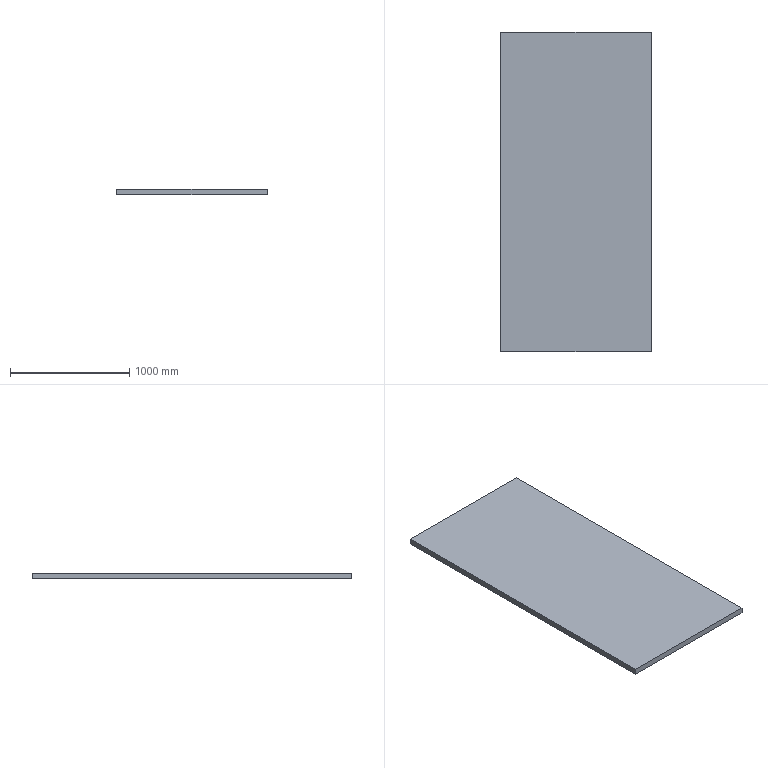Part | STEP file | 1 solid | 6 faces | box 1260 x 2677 x 50 mm | volume 168683678 mm3 | plane 6
STEP:
#1=CARTESIAN_POINT('',(0.,0.,0.));
#2=DIRECTION('',(0.,0.,1.));
#3=DIRECTION('',(1.,0.,0.));
#4=AXIS2_PLACEMENT_3D('',#1,#2,#3);
#5=CARTESIAN_POINT('',(6051.871,-1690.161,-25.));
#6=VERTEX_POINT('',#5);
#7=CARTESIAN_POINT('',(6051.871,986.805,-25.));
#8=VERTEX_POINT('',#7);
#9=CARTESIAN_POINT('',(6051.871,986.805,-25.));
#10=DIRECTION('',(0.,1.,0.));
#11=VECTOR('',#10,1.);
#12=LINE('',#9,#11);
#13=CARTESIAN_POINT('',(6051.871,986.805,25.));
#14=DIRECTION('',(-1.,0.,0.));
#15=DIRECTION('',(0.,0.,1.));
#16=AXIS2_PLACEMENT_3D('',#13,#14,#15);
#17=PLANE('',#16);
#18=CARTESIAN_POINT('',(-50.,0.));
#19=DIRECTION('',(0.,1.));
#20=VECTOR('',#19,1.);
#21=LINE('',#18,#20);
#22=(GEOMETRIC_REPRESENTATION_CONTEXT(2)PARAMETRIC_REPRESENTATION_CONTEXT()REPRESENTATION_CONTEXT('',''));
#23=DEFINITIONAL_REPRESENTATION('',(#21),#22);
#24=PCURVE('',#17,#23);
#25=CARTESIAN_POINT('',(0.,0.,-25.));
#26=DIRECTION('',(0.,0.,-1.));
#27=DIRECTION('',(-1.,0.,0.));
#28=AXIS2_PLACEMENT_3D('',#25,#26,#27);
#29=PLANE('',#28);
#30=CARTESIAN_POINT('',(-6051.871,986.805));
#31=DIRECTION('',(0.,1.));
#32=VECTOR('',#31,1.);
#33=LINE('',#30,#32);
#34=(GEOMETRIC_REPRESENTATION_CONTEXT(2)PARAMETRIC_REPRESENTATION_CONTEXT()REPRESENTATION_CONTEXT('',''));
#35=DEFINITIONAL_REPRESENTATION('',(#33),#34);
#36=PCURVE('',#29,#35);
#37=SURFACE_CURVE('',#12,(#24,#36),.PCURVE_S1.);
#38=EDGE_CURVE('',#6,#8,#37,.T.);
#39=ORIENTED_EDGE('',*,*,#38,.T.);
#40=CARTESIAN_POINT('',(6051.871,986.805,25.));
#41=VERTEX_POINT('',#40);
#42=CARTESIAN_POINT('',(6051.871,986.805,25.));
#43=DIRECTION('',(0.,0.,-1.));
#44=VECTOR('',#43,1.);
#45=LINE('',#42,#44);
#46=CARTESIAN_POINT('',(0.,0.));
#47=DIRECTION('',(-1.,0.));
#48=VECTOR('',#47,1.);
#49=LINE('',#46,#48);
#50=(GEOMETRIC_REPRESENTATION_CONTEXT(2)PARAMETRIC_REPRESENTATION_CONTEXT()REPRESENTATION_CONTEXT('',''));
#51=DEFINITIONAL_REPRESENTATION('',(#49),#50);
#52=PCURVE('',#17,#51);
#53=CARTESIAN_POINT('',(6051.871,986.805,25.));
#54=DIRECTION('',(0.,-1.,0.));
#55=DIRECTION('',(0.,0.,-1.));
#56=AXIS2_PLACEMENT_3D('',#53,#54,#55);
#57=PLANE('',#56);
#58=CARTESIAN_POINT('',(0.,0.));
#59=DIRECTION('',(1.,0.));
#60=VECTOR('',#59,1.);
#61=LINE('',#58,#60);
#62=(GEOMETRIC_REPRESENTATION_CONTEXT(2)PARAMETRIC_REPRESENTATION_CONTEXT()REPRESENTATION_CONTEXT('',''));
#63=DEFINITIONAL_REPRESENTATION('',(#61),#62);
#64=PCURVE('',#57,#63);
#65=SURFACE_CURVE('',#45,(#52,#64),.PCURVE_S1.);
#66=EDGE_CURVE('',#41,#8,#65,.T.);
#67=ORIENTED_EDGE('',*,*,#66,.F.);
#68=CARTESIAN_POINT('',(6051.871,-1690.161,25.));
#69=VERTEX_POINT('',#68);
#70=CARTESIAN_POINT('',(6051.871,986.805,25.));
#71=DIRECTION('',(0.,1.,0.));
#72=VECTOR('',#71,1.);
#73=LINE('',#70,#72);
#74=CARTESIAN_POINT('',(0.,0.));
#75=DIRECTION('',(0.,1.));
#76=VECTOR('',#75,1.);
#77=LINE('',#74,#76);
#78=(GEOMETRIC_REPRESENTATION_CONTEXT(2)PARAMETRIC_REPRESENTATION_CONTEXT()REPRESENTATION_CONTEXT('',''));
#79=DEFINITIONAL_REPRESENTATION('',(#77),#78);
#80=PCURVE('',#17,#79);
#81=CARTESIAN_POINT('',(0.,0.,25.));
#82=DIRECTION('',(0.,0.,-1.));
#83=DIRECTION('',(-1.,0.,0.));
#84=AXIS2_PLACEMENT_3D('',#81,#82,#83);
#85=PLANE('',#84);
#86=CARTESIAN_POINT('',(-6051.871,986.805));
#87=DIRECTION('',(0.,1.));
#88=VECTOR('',#87,1.);
#89=LINE('',#86,#88);
#90=(GEOMETRIC_REPRESENTATION_CONTEXT(2)PARAMETRIC_REPRESENTATION_CONTEXT()REPRESENTATION_CONTEXT('',''));
#91=DEFINITIONAL_REPRESENTATION('',(#89),#90);
#92=PCURVE('',#85,#91);
#93=SURFACE_CURVE('',#73,(#80,#92),.PCURVE_S1.);
#94=EDGE_CURVE('',#69,#41,#93,.T.);
#95=ORIENTED_EDGE('',*,*,#94,.F.);
#96=CARTESIAN_POINT('',(6051.871,-1690.161,25.));
#97=DIRECTION('',(0.,0.,-1.));
#98=VECTOR('',#97,1.);
#99=LINE('',#96,#98);
#100=CARTESIAN_POINT('',(0.,-2676.966));
#101=DIRECTION('',(-1.,0.));
#102=VECTOR('',#101,1.);
#103=LINE('',#100,#102);
#104=(GEOMETRIC_REPRESENTATION_CONTEXT(2)PARAMETRIC_REPRESENTATION_CONTEXT()REPRESENTATION_CONTEXT('',''));
#105=DEFINITIONAL_REPRESENTATION('',(#103),#104);
#106=PCURVE('',#17,#105);
#107=CARTESIAN_POINT('',(6051.871,-1690.161,25.));
#108=DIRECTION('',(0.,1.,0.));
#109=DIRECTION('',(0.,0.,1.));
#110=AXIS2_PLACEMENT_3D('',#107,#108,#109);
#111=PLANE('',#110);
#112=CARTESIAN_POINT('',(0.,0.));
#113=DIRECTION('',(-1.,0.));
#114=VECTOR('',#113,1.);
#115=LINE('',#112,#114);
#116=(GEOMETRIC_REPRESENTATION_CONTEXT(2)PARAMETRIC_REPRESENTATION_CONTEXT()REPRESENTATION_CONTEXT('',''));
#117=DEFINITIONAL_REPRESENTATION('',(#115),#116);
#118=PCURVE('',#111,#117);
#119=SURFACE_CURVE('',#99,(#106,#118),.PCURVE_S1.);
#120=EDGE_CURVE('',#69,#6,#119,.T.);
#121=ORIENTED_EDGE('',*,*,#120,.T.);
#122=EDGE_LOOP('',(#39,#67,#95,#121));
#123=FACE_BOUND('',#122,.T.);
#124=ADVANCED_FACE('',(#123),#17,.F.);
#125=CARTESIAN_POINT('',(4791.611,986.805,-25.));
#126=VERTEX_POINT('',#125);
#127=CARTESIAN_POINT('',(6051.871,986.805,-25.));
#128=DIRECTION('',(-1.,0.,0.));
#129=VECTOR('',#128,1.);
#130=LINE('',#127,#129);
#131=CARTESIAN_POINT('',(50.,0.));
#132=DIRECTION('',(0.,-1.));
#133=VECTOR('',#132,1.);
#134=LINE('',#131,#133);
#135=(GEOMETRIC_REPRESENTATION_CONTEXT(2)PARAMETRIC_REPRESENTATION_CONTEXT()REPRESENTATION_CONTEXT('',''));
#136=DEFINITIONAL_REPRESENTATION('',(#134),#135);
#137=PCURVE('',#57,#136);
#138=CARTESIAN_POINT('',(-6051.871,986.805));
#139=DIRECTION('',(1.,0.));
#140=VECTOR('',#139,1.);
#141=LINE('',#138,#140);
#142=(GEOMETRIC_REPRESENTATION_CONTEXT(2)PARAMETRIC_REPRESENTATION_CONTEXT()REPRESENTATION_CONTEXT('',''));
#143=DEFINITIONAL_REPRESENTATION('',(#141),#142);
#144=PCURVE('',#29,#143);
#145=SURFACE_CURVE('',#130,(#137,#144),.PCURVE_S1.);
#146=EDGE_CURVE('',#8,#126,#145,.T.);
#147=ORIENTED_EDGE('',*,*,#146,.T.);
#148=CARTESIAN_POINT('',(4791.611,986.805,25.));
#149=VERTEX_POINT('',#148);
#150=CARTESIAN_POINT('',(4791.611,986.805,25.));
#151=DIRECTION('',(0.,0.,-1.));
#152=VECTOR('',#151,1.);
#153=LINE('',#150,#152);
#154=CARTESIAN_POINT('',(0.,-1260.26));
#155=DIRECTION('',(1.,0.));
#156=VECTOR('',#155,1.);
#157=LINE('',#154,#156);
#158=(GEOMETRIC_REPRESENTATION_CONTEXT(2)PARAMETRIC_REPRESENTATION_CONTEXT()REPRESENTATION_CONTEXT('',''));
#159=DEFINITIONAL_REPRESENTATION('',(#157),#158);
#160=PCURVE('',#57,#159);
#161=CARTESIAN_POINT('',(4791.611,986.805,25.));
#162=DIRECTION('',(1.,0.,0.));
#163=DIRECTION('',(0.,0.,-1.));
#164=AXIS2_PLACEMENT_3D('',#161,#162,#163);
#165=PLANE('',#164);
#166=CARTESIAN_POINT('',(0.,0.));
#167=DIRECTION('',(1.,0.));
#168=VECTOR('',#167,1.);
#169=LINE('',#166,#168);
#170=(GEOMETRIC_REPRESENTATION_CONTEXT(2)PARAMETRIC_REPRESENTATION_CONTEXT()REPRESENTATION_CONTEXT('',''));
#171=DEFINITIONAL_REPRESENTATION('',(#169),#170);
#172=PCURVE('',#165,#171);
#173=SURFACE_CURVE('',#153,(#160,#172),.PCURVE_S1.);
#174=EDGE_CURVE('',#149,#126,#173,.T.);
#175=ORIENTED_EDGE('',*,*,#174,.F.);
#176=CARTESIAN_POINT('',(6051.871,986.805,25.));
#177=DIRECTION('',(-1.,0.,0.));
#178=VECTOR('',#177,1.);
#179=LINE('',#176,#178);
#180=CARTESIAN_POINT('',(0.,0.));
#181=DIRECTION('',(0.,-1.));
#182=VECTOR('',#181,1.);
#183=LINE('',#180,#182);
#184=(GEOMETRIC_REPRESENTATION_CONTEXT(2)PARAMETRIC_REPRESENTATION_CONTEXT()REPRESENTATION_CONTEXT('',''));
#185=DEFINITIONAL_REPRESENTATION('',(#183),#184);
#186=PCURVE('',#57,#185);
#187=CARTESIAN_POINT('',(-6051.871,986.805));
#188=DIRECTION('',(1.,0.));
#189=VECTOR('',#188,1.);
#190=LINE('',#187,#189);
#191=(GEOMETRIC_REPRESENTATION_CONTEXT(2)PARAMETRIC_REPRESENTATION_CONTEXT()REPRESENTATION_CONTEXT('',''));
#192=DEFINITIONAL_REPRESENTATION('',(#190),#191);
#193=PCURVE('',#85,#192);
#194=SURFACE_CURVE('',#179,(#186,#193),.PCURVE_S1.);
#195=EDGE_CURVE('',#41,#149,#194,.T.);
#196=ORIENTED_EDGE('',*,*,#195,.F.);
#197=ORIENTED_EDGE('',*,*,#66,.T.);
#198=EDGE_LOOP('',(#147,#175,#196,#197));
#199=FACE_BOUND('',#198,.T.);
#200=ADVANCED_FACE('',(#199),#57,.F.);
#201=CARTESIAN_POINT('',(4791.611,-1690.161,-25.));
#202=VERTEX_POINT('',#201);
#203=CARTESIAN_POINT('',(4791.611,986.805,-25.));
#204=DIRECTION('',(0.,-1.,0.));
#205=VECTOR('',#204,1.);
#206=LINE('',#203,#205);
#207=CARTESIAN_POINT('',(50.,0.));
#208=DIRECTION('',(0.,-1.));
#209=VECTOR('',#208,1.);
#210=LINE('',#207,#209);
#211=(GEOMETRIC_REPRESENTATION_CONTEXT(2)PARAMETRIC_REPRESENTATION_CONTEXT()REPRESENTATION_CONTEXT('',''));
#212=DEFINITIONAL_REPRESENTATION('',(#210),#211);
#213=PCURVE('',#165,#212);
#214=CARTESIAN_POINT('',(-4791.611,986.805));
#215=DIRECTION('',(0.,-1.));
#216=VECTOR('',#215,1.);
#217=LINE('',#214,#216);
#218=(GEOMETRIC_REPRESENTATION_CONTEXT(2)PARAMETRIC_REPRESENTATION_CONTEXT()REPRESENTATION_CONTEXT('',''));
#219=DEFINITIONAL_REPRESENTATION('',(#217),#218);
#220=PCURVE('',#29,#219);
#221=SURFACE_CURVE('',#206,(#213,#220),.PCURVE_S1.);
#222=EDGE_CURVE('',#126,#202,#221,.T.);
#223=ORIENTED_EDGE('',*,*,#222,.T.);
#224=CARTESIAN_POINT('',(4791.611,-1690.161,25.));
#225=VERTEX_POINT('',#224);
#226=CARTESIAN_POINT('',(4791.611,-1690.161,25.));
#227=DIRECTION('',(0.,0.,-1.));
#228=VECTOR('',#227,1.);
#229=LINE('',#226,#228);
#230=CARTESIAN_POINT('',(0.,-2676.966));
#231=DIRECTION('',(1.,0.));
#232=VECTOR('',#231,1.);
#233=LINE('',#230,#232);
#234=(GEOMETRIC_REPRESENTATION_CONTEXT(2)PARAMETRIC_REPRESENTATION_CONTEXT()REPRESENTATION_CONTEXT('',''));
#235=DEFINITIONAL_REPRESENTATION('',(#233),#234);
#236=PCURVE('',#165,#235);
#237=CARTESIAN_POINT('',(0.,-1260.26));
#238=DIRECTION('',(-1.,0.));
#239=VECTOR('',#238,1.);
#240=LINE('',#237,#239);
#241=(GEOMETRIC_REPRESENTATION_CONTEXT(2)PARAMETRIC_REPRESENTATION_CONTEXT()REPRESENTATION_CONTEXT('',''));
#242=DEFINITIONAL_REPRESENTATION('',(#240),#241);
#243=PCURVE('',#111,#242);
#244=SURFACE_CURVE('',#229,(#236,#243),.PCURVE_S1.);
#245=EDGE_CURVE('',#225,#202,#244,.T.);
#246=ORIENTED_EDGE('',*,*,#245,.F.);
#247=CARTESIAN_POINT('',(4791.611,986.805,25.));
#248=DIRECTION('',(0.,-1.,0.));
#249=VECTOR('',#248,1.);
#250=LINE('',#247,#249);
#251=CARTESIAN_POINT('',(0.,0.));
#252=DIRECTION('',(0.,-1.));
#253=VECTOR('',#252,1.);
#254=LINE('',#251,#253);
#255=(GEOMETRIC_REPRESENTATION_CONTEXT(2)PARAMETRIC_REPRESENTATION_CONTEXT()REPRESENTATION_CONTEXT('',''));
#256=DEFINITIONAL_REPRESENTATION('',(#254),#255);
#257=PCURVE('',#165,#256);
#258=CARTESIAN_POINT('',(-4791.611,986.805));
#259=DIRECTION('',(0.,-1.));
#260=VECTOR('',#259,1.);
#261=LINE('',#258,#260);
#262=(GEOMETRIC_REPRESENTATION_CONTEXT(2)PARAMETRIC_REPRESENTATION_CONTEXT()REPRESENTATION_CONTEXT('',''));
#263=DEFINITIONAL_REPRESENTATION('',(#261),#262);
#264=PCURVE('',#85,#263);
#265=SURFACE_CURVE('',#250,(#257,#264),.PCURVE_S1.);
#266=EDGE_CURVE('',#149,#225,#265,.T.);
#267=ORIENTED_EDGE('',*,*,#266,.F.);
#268=ORIENTED_EDGE('',*,*,#174,.T.);
#269=EDGE_LOOP('',(#223,#246,#267,#268));
#270=FACE_BOUND('',#269,.T.);
#271=ADVANCED_FACE('',(#270),#165,.F.);
#272=CARTESIAN_POINT('',(6051.871,-1690.161,-25.));
#273=DIRECTION('',(1.,0.,0.));
#274=VECTOR('',#273,1.);
#275=LINE('',#272,#274);
#276=CARTESIAN_POINT('',(-50.,0.));
#277=DIRECTION('',(0.,1.));
#278=VECTOR('',#277,1.);
#279=LINE('',#276,#278);
#280=(GEOMETRIC_REPRESENTATION_CONTEXT(2)PARAMETRIC_REPRESENTATION_CONTEXT()REPRESENTATION_CONTEXT('',''));
#281=DEFINITIONAL_REPRESENTATION('',(#279),#280);
#282=PCURVE('',#111,#281);
#283=CARTESIAN_POINT('',(-6051.871,-1690.161));
#284=DIRECTION('',(-1.,0.));
#285=VECTOR('',#284,1.);
#286=LINE('',#283,#285);
#287=(GEOMETRIC_REPRESENTATION_CONTEXT(2)PARAMETRIC_REPRESENTATION_CONTEXT()REPRESENTATION_CONTEXT('',''));
#288=DEFINITIONAL_REPRESENTATION('',(#286),#287);
#289=PCURVE('',#29,#288);
#290=SURFACE_CURVE('',#275,(#282,#289),.PCURVE_S1.);
#291=EDGE_CURVE('',#202,#6,#290,.T.);
#292=ORIENTED_EDGE('',*,*,#291,.T.);
#293=ORIENTED_EDGE('',*,*,#120,.F.);
#294=CARTESIAN_POINT('',(6051.871,-1690.161,25.));
#295=DIRECTION('',(1.,0.,0.));
#296=VECTOR('',#295,1.);
#297=LINE('',#294,#296);
#298=CARTESIAN_POINT('',(0.,0.));
#299=DIRECTION('',(0.,1.));
#300=VECTOR('',#299,1.);
#301=LINE('',#298,#300);
#302=(GEOMETRIC_REPRESENTATION_CONTEXT(2)PARAMETRIC_REPRESENTATION_CONTEXT()REPRESENTATION_CONTEXT('',''));
#303=DEFINITIONAL_REPRESENTATION('',(#301),#302);
#304=PCURVE('',#111,#303);
#305=CARTESIAN_POINT('',(-6051.871,-1690.161));
#306=DIRECTION('',(-1.,0.));
#307=VECTOR('',#306,1.);
#308=LINE('',#305,#307);
#309=(GEOMETRIC_REPRESENTATION_CONTEXT(2)PARAMETRIC_REPRESENTATION_CONTEXT()REPRESENTATION_CONTEXT('',''));
#310=DEFINITIONAL_REPRESENTATION('',(#308),#309);
#311=PCURVE('',#85,#310);
#312=SURFACE_CURVE('',#297,(#304,#311),.PCURVE_S1.);
#313=EDGE_CURVE('',#225,#69,#312,.T.);
#314=ORIENTED_EDGE('',*,*,#313,.F.);
#315=ORIENTED_EDGE('',*,*,#245,.T.);
#316=EDGE_LOOP('',(#292,#293,#314,#315));
#317=FACE_BOUND('',#316,.T.);
#318=ADVANCED_FACE('',(#317),#111,.F.);
#319=ORIENTED_EDGE('',*,*,#94,.T.);
#320=ORIENTED_EDGE('',*,*,#195,.T.);
#321=ORIENTED_EDGE('',*,*,#266,.T.);
#322=ORIENTED_EDGE('',*,*,#313,.T.);
#323=EDGE_LOOP('',(#319,#320,#321,#322));
#324=FACE_BOUND('',#323,.T.);
#325=ADVANCED_FACE('',(#324),#85,.F.);
#326=ORIENTED_EDGE('',*,*,#38,.F.);
#327=ORIENTED_EDGE('',*,*,#291,.F.);
#328=ORIENTED_EDGE('',*,*,#222,.F.);
#329=ORIENTED_EDGE('',*,*,#146,.F.);
#330=EDGE_LOOP('',(#326,#327,#328,#329));
#331=FACE_BOUND('',#330,.T.);
#332=ADVANCED_FACE('',(#331),#29,.T.);
#333=CLOSED_SHELL('',(#124,#200,#271,#318,#325,#332));
#334=MANIFOLD_SOLID_BREP('',#333);
#335=(LENGTH_UNIT()NAMED_UNIT(*)SI_UNIT(.MILLI.,.METRE.));
#336=UNCERTAINTY_MEASURE_WITH_UNIT(LENGTH_MEASURE(0.0000001),#335,'','');
#337=(NAMED_UNIT(*)PLANE_ANGLE_UNIT()SI_UNIT($,.RADIAN.));
#338=(NAMED_UNIT(*)SI_UNIT($,.STERADIAN.)SOLID_ANGLE_UNIT());
#339=(GEOMETRIC_REPRESENTATION_CONTEXT(3)GLOBAL_UNCERTAINTY_ASSIGNED_CONTEXT((#336))GLOBAL_UNIT_ASSIGNED_CONTEXT((#335,#337,#338))REPRESENTATION_CONTEXT('',''));
#340=ADVANCED_BREP_SHAPE_REPRESENTATION('',(#4,#334),#339);